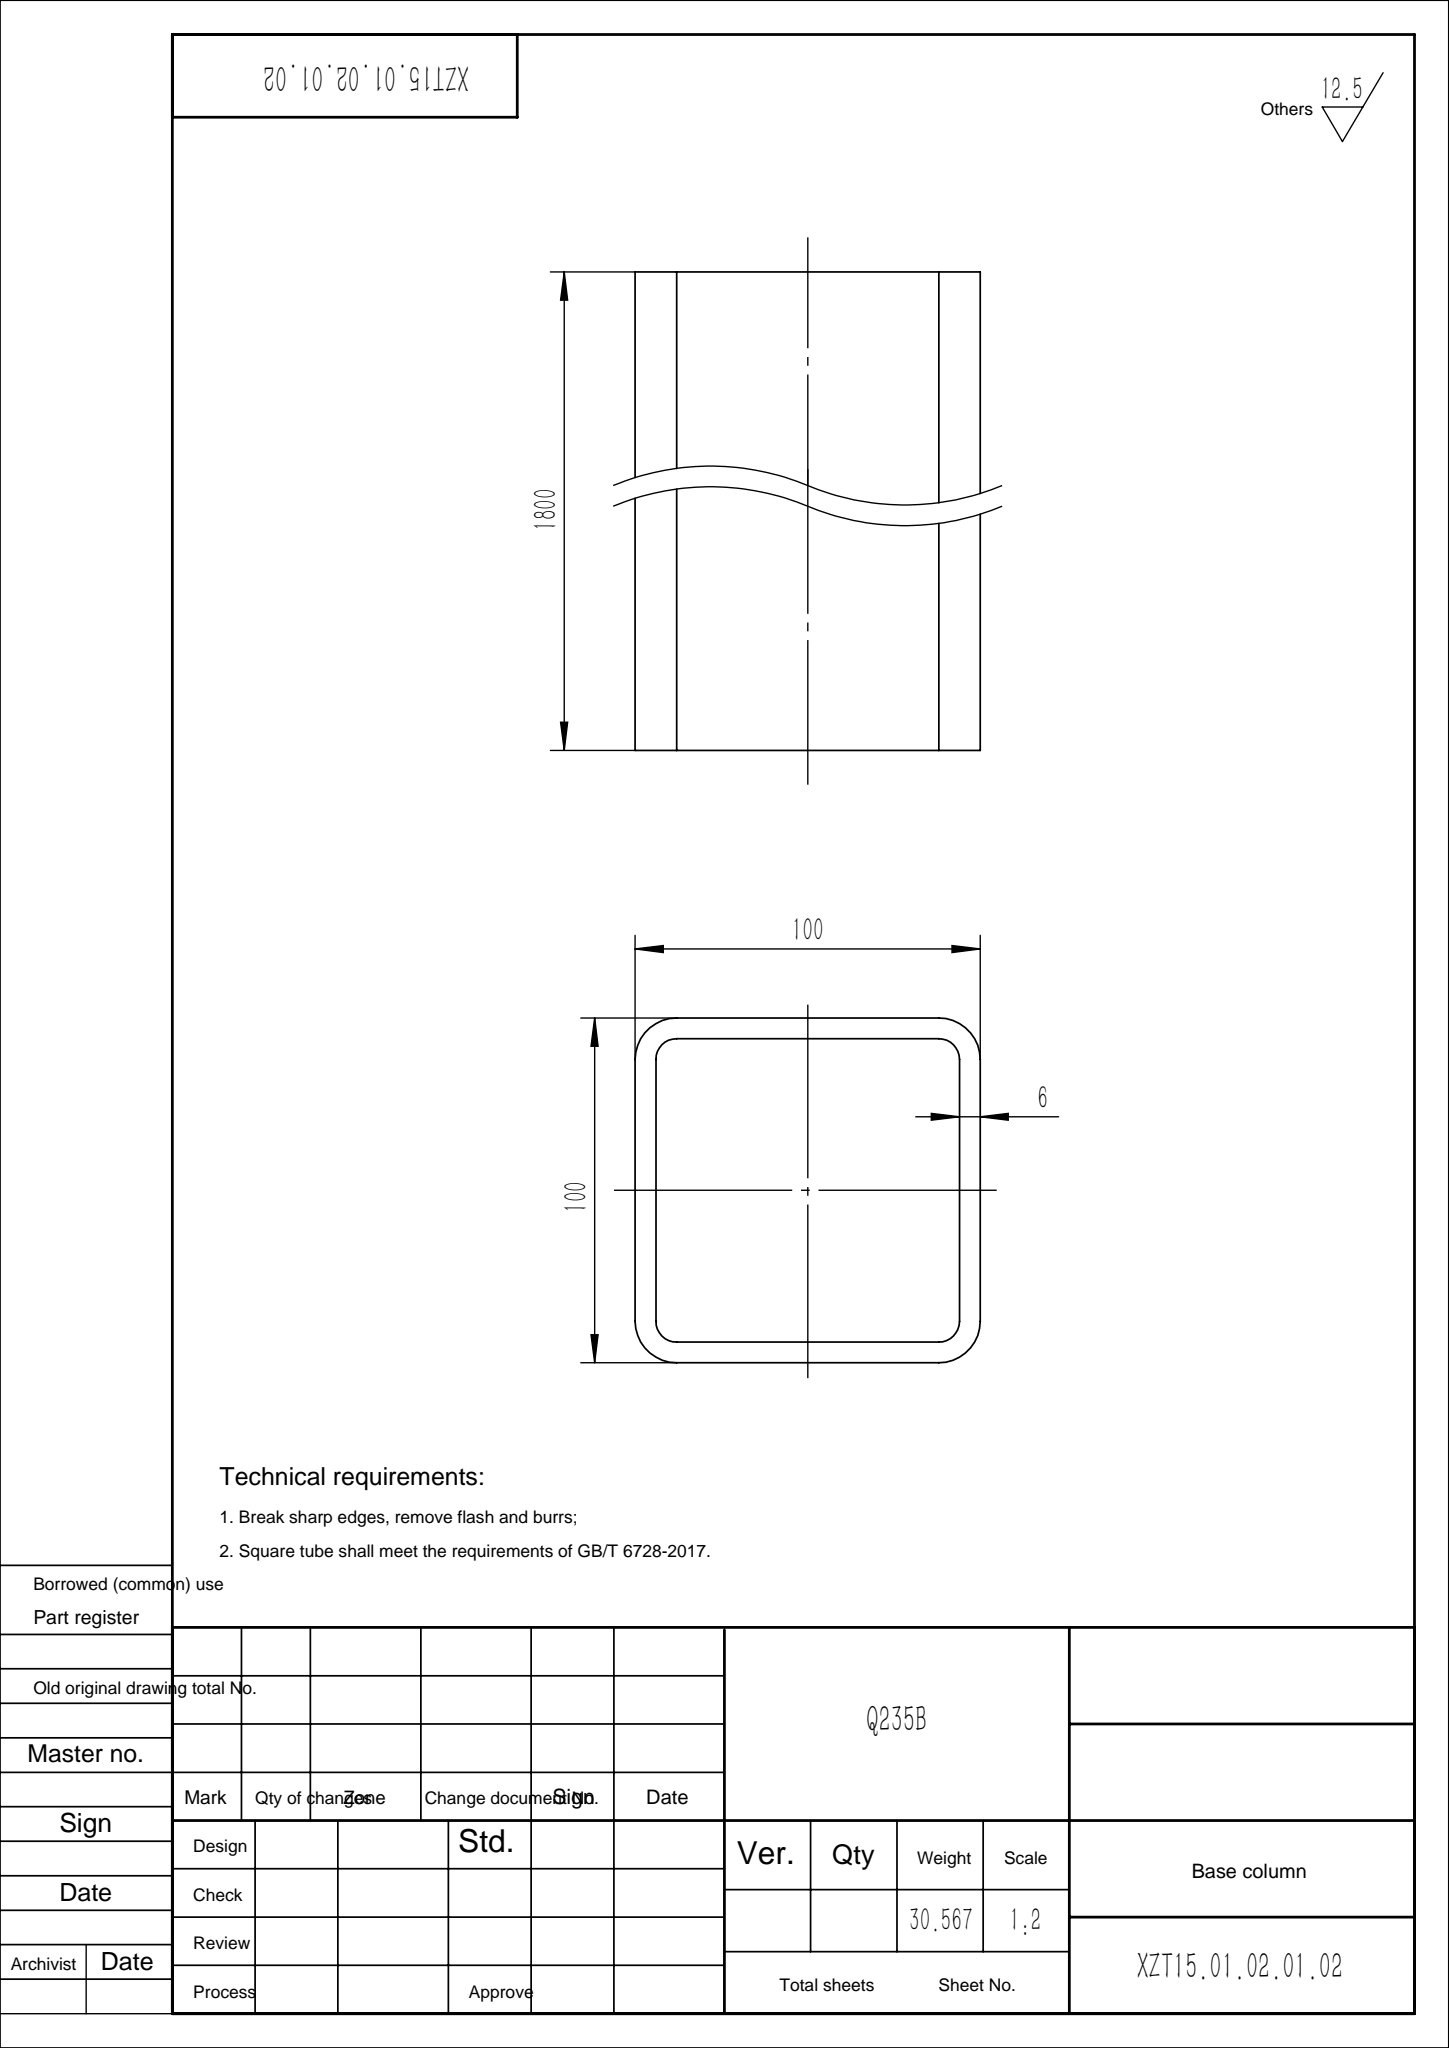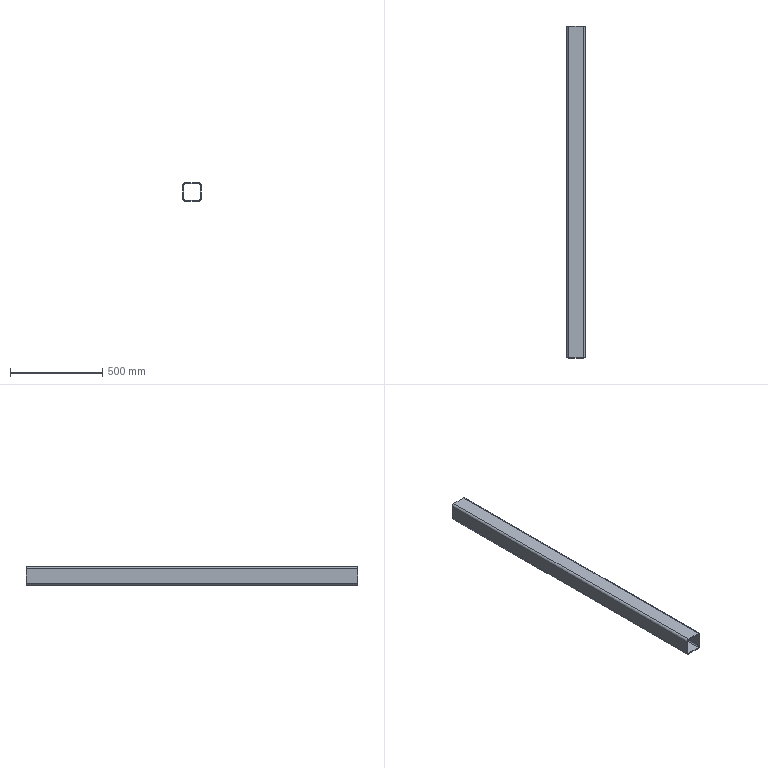Part | SolidWorks | features WeldMemberFeat 1, WeldmentFeature 1 | 1 solid | 18 faces | box 100 x 1800 x 100 mm | volume 3893926 mm3 | plane 10 | cylinder 8 | commonest cylinder face diameters 12 x4 24 x4
STEP:
#1=CARTESIAN_POINT('',(-50.,0.,38.));
#2=VERTEX_POINT('',#1);
#3=CARTESIAN_POINT('',(-38.,0.,50.));
#4=VERTEX_POINT('',#3);
#5=CARTESIAN_POINT('',(-38.,0.,38.));
#6=DIRECTION('',(0.,1.,0.));
#7=DIRECTION('',(0.,0.,1.));
#8=AXIS2_PLACEMENT_3D('',#5,#6,#7);
#9=CIRCLE('',#8,12.);
#10=EDGE_CURVE('',#2,#4,#9,.T.);
#11=ORIENTED_EDGE('',*,*,#10,.T.);
#12=CARTESIAN_POINT('',(-38.,1800.,50.));
#13=VERTEX_POINT('',#12);
#14=CARTESIAN_POINT('',(-38.,1800.,50.));
#15=DIRECTION('',(0.,-1.,0.));
#16=VECTOR('',#15,1000.);
#17=LINE('',#14,#16);
#18=EDGE_CURVE('',#13,#4,#17,.T.);
#19=ORIENTED_EDGE('',*,*,#18,.F.);
#20=CARTESIAN_POINT('',(-50.,1800.,38.));
#21=VERTEX_POINT('',#20);
#22=CARTESIAN_POINT('',(-38.,1800.,38.));
#23=DIRECTION('',(0.,1.,0.));
#24=DIRECTION('',(0.,0.,1.));
#25=AXIS2_PLACEMENT_3D('',#22,#23,#24);
#26=CIRCLE('',#25,12.);
#27=EDGE_CURVE('',#21,#13,#26,.T.);
#28=ORIENTED_EDGE('',*,*,#27,.F.);
#29=CARTESIAN_POINT('',(-50.,1800.,38.));
#30=DIRECTION('',(0.,-1.,0.));
#31=VECTOR('',#30,1000.);
#32=LINE('',#29,#31);
#33=EDGE_CURVE('',#21,#2,#32,.T.);
#34=ORIENTED_EDGE('',*,*,#33,.T.);
#35=EDGE_LOOP('',(#11,#19,#28,#34));
#36=FACE_OUTER_BOUND('',#35,.T.);
#37=CARTESIAN_POINT('',(-38.,1800.,38.));
#38=DIRECTION('',(0.,-1.,0.));
#39=DIRECTION('',(0.,0.,-1.));
#40=AXIS2_PLACEMENT_3D('',#37,#38,#39);
#41=CYLINDRICAL_SURFACE('',#40,12.);
#42=ADVANCED_FACE('',(#36),#41,.T.);
#43=CARTESIAN_POINT('',(38.,0.,50.));
#44=VERTEX_POINT('',#43);
#45=CARTESIAN_POINT('',(-38.,0.,50.));
#46=DIRECTION('',(1.,0.,0.));
#47=VECTOR('',#46,1000.);
#48=LINE('',#45,#47);
#49=EDGE_CURVE('',#4,#44,#48,.T.);
#50=ORIENTED_EDGE('',*,*,#49,.T.);
#51=CARTESIAN_POINT('',(38.,1800.,50.));
#52=VERTEX_POINT('',#51);
#53=CARTESIAN_POINT('',(38.,1800.,50.));
#54=DIRECTION('',(0.,-1.,0.));
#55=VECTOR('',#54,1000.);
#56=LINE('',#53,#55);
#57=EDGE_CURVE('',#52,#44,#56,.T.);
#58=ORIENTED_EDGE('',*,*,#57,.F.);
#59=CARTESIAN_POINT('',(-38.,1800.,50.));
#60=DIRECTION('',(1.,0.,0.));
#61=VECTOR('',#60,1000.);
#62=LINE('',#59,#61);
#63=EDGE_CURVE('',#13,#52,#62,.T.);
#64=ORIENTED_EDGE('',*,*,#63,.F.);
#65=ORIENTED_EDGE('',*,*,#18,.T.);
#66=EDGE_LOOP('',(#50,#58,#64,#65));
#67=FACE_OUTER_BOUND('',#66,.T.);
#68=CARTESIAN_POINT('',(-38.,1800.,50.));
#69=DIRECTION('',(0.,0.,-1.));
#70=DIRECTION('',(-1.,0.,0.));
#71=AXIS2_PLACEMENT_3D('',#68,#69,#70);
#72=PLANE('',#71);
#73=ADVANCED_FACE('',(#67),#72,.F.);
#74=CARTESIAN_POINT('',(50.,0.,38.));
#75=VERTEX_POINT('',#74);
#76=CARTESIAN_POINT('',(38.,0.,38.));
#77=DIRECTION('',(0.,1.,0.));
#78=DIRECTION('',(0.,0.,1.));
#79=AXIS2_PLACEMENT_3D('',#76,#77,#78);
#80=CIRCLE('',#79,12.);
#81=EDGE_CURVE('',#44,#75,#80,.T.);
#82=ORIENTED_EDGE('',*,*,#81,.T.);
#83=CARTESIAN_POINT('',(50.,1800.,38.));
#84=VERTEX_POINT('',#83);
#85=CARTESIAN_POINT('',(50.,1800.,38.));
#86=DIRECTION('',(0.,-1.,0.));
#87=VECTOR('',#86,1000.);
#88=LINE('',#85,#87);
#89=EDGE_CURVE('',#84,#75,#88,.T.);
#90=ORIENTED_EDGE('',*,*,#89,.F.);
#91=CARTESIAN_POINT('',(38.,1800.,38.));
#92=DIRECTION('',(0.,1.,0.));
#93=DIRECTION('',(0.,0.,1.));
#94=AXIS2_PLACEMENT_3D('',#91,#92,#93);
#95=CIRCLE('',#94,12.);
#96=EDGE_CURVE('',#52,#84,#95,.T.);
#97=ORIENTED_EDGE('',*,*,#96,.F.);
#98=ORIENTED_EDGE('',*,*,#57,.T.);
#99=EDGE_LOOP('',(#82,#90,#97,#98));
#100=FACE_OUTER_BOUND('',#99,.T.);
#101=CARTESIAN_POINT('',(38.,1800.,38.));
#102=DIRECTION('',(0.,-1.,0.));
#103=DIRECTION('',(0.,0.,-1.));
#104=AXIS2_PLACEMENT_3D('',#101,#102,#103);
#105=CYLINDRICAL_SURFACE('',#104,12.);
#106=ADVANCED_FACE('',(#100),#105,.T.);
#107=CARTESIAN_POINT('',(50.,0.,-38.));
#108=VERTEX_POINT('',#107);
#109=CARTESIAN_POINT('',(50.,0.,-38.));
#110=DIRECTION('',(0.,0.,-1.));
#111=VECTOR('',#110,1000.);
#112=LINE('',#109,#111);
#113=EDGE_CURVE('',#75,#108,#112,.T.);
#114=ORIENTED_EDGE('',*,*,#113,.T.);
#115=CARTESIAN_POINT('',(50.,1800.,-38.));
#116=VERTEX_POINT('',#115);
#117=CARTESIAN_POINT('',(50.,1800.,-38.));
#118=DIRECTION('',(0.,-1.,0.));
#119=VECTOR('',#118,1000.);
#120=LINE('',#117,#119);
#121=EDGE_CURVE('',#116,#108,#120,.T.);
#122=ORIENTED_EDGE('',*,*,#121,.F.);
#123=CARTESIAN_POINT('',(50.,1800.,-38.));
#124=DIRECTION('',(0.,0.,-1.));
#125=VECTOR('',#124,1000.);
#126=LINE('',#123,#125);
#127=EDGE_CURVE('',#84,#116,#126,.T.);
#128=ORIENTED_EDGE('',*,*,#127,.F.);
#129=ORIENTED_EDGE('',*,*,#89,.T.);
#130=EDGE_LOOP('',(#114,#122,#128,#129));
#131=FACE_OUTER_BOUND('',#130,.T.);
#132=CARTESIAN_POINT('',(50.,1800.,-38.));
#133=DIRECTION('',(-1.,0.,0.));
#134=DIRECTION('',(0.,0.,1.));
#135=AXIS2_PLACEMENT_3D('',#132,#133,#134);
#136=PLANE('',#135);
#137=ADVANCED_FACE('',(#131),#136,.F.);
#138=CARTESIAN_POINT('',(38.,0.,-50.));
#139=VERTEX_POINT('',#138);
#140=CARTESIAN_POINT('',(38.,0.,-38.));
#141=DIRECTION('',(0.,1.,0.));
#142=DIRECTION('',(0.,0.,1.));
#143=AXIS2_PLACEMENT_3D('',#140,#141,#142);
#144=CIRCLE('',#143,12.);
#145=EDGE_CURVE('',#108,#139,#144,.T.);
#146=ORIENTED_EDGE('',*,*,#145,.T.);
#147=CARTESIAN_POINT('',(38.,1800.,-50.));
#148=VERTEX_POINT('',#147);
#149=CARTESIAN_POINT('',(38.,1800.,-50.));
#150=DIRECTION('',(0.,-1.,0.));
#151=VECTOR('',#150,1000.);
#152=LINE('',#149,#151);
#153=EDGE_CURVE('',#148,#139,#152,.T.);
#154=ORIENTED_EDGE('',*,*,#153,.F.);
#155=CARTESIAN_POINT('',(38.,1800.,-38.));
#156=DIRECTION('',(0.,1.,0.));
#157=DIRECTION('',(0.,0.,1.));
#158=AXIS2_PLACEMENT_3D('',#155,#156,#157);
#159=CIRCLE('',#158,12.);
#160=EDGE_CURVE('',#116,#148,#159,.T.);
#161=ORIENTED_EDGE('',*,*,#160,.F.);
#162=ORIENTED_EDGE('',*,*,#121,.T.);
#163=EDGE_LOOP('',(#146,#154,#161,#162));
#164=FACE_OUTER_BOUND('',#163,.T.);
#165=CARTESIAN_POINT('',(38.,1800.,-38.));
#166=DIRECTION('',(0.,-1.,0.));
#167=DIRECTION('',(0.,0.,-1.));
#168=AXIS2_PLACEMENT_3D('',#165,#166,#167);
#169=CYLINDRICAL_SURFACE('',#168,12.);
#170=ADVANCED_FACE('',(#164),#169,.T.);
#171=CARTESIAN_POINT('',(-38.,0.,-50.));
#172=VERTEX_POINT('',#171);
#173=CARTESIAN_POINT('',(38.,0.,-50.));
#174=DIRECTION('',(-1.,0.,0.));
#175=VECTOR('',#174,1000.);
#176=LINE('',#173,#175);
#177=EDGE_CURVE('',#139,#172,#176,.T.);
#178=ORIENTED_EDGE('',*,*,#177,.T.);
#179=CARTESIAN_POINT('',(-38.,1800.,-50.));
#180=VERTEX_POINT('',#179);
#181=CARTESIAN_POINT('',(-38.,1800.,-50.));
#182=DIRECTION('',(0.,-1.,0.));
#183=VECTOR('',#182,1000.);
#184=LINE('',#181,#183);
#185=EDGE_CURVE('',#180,#172,#184,.T.);
#186=ORIENTED_EDGE('',*,*,#185,.F.);
#187=CARTESIAN_POINT('',(38.,1800.,-50.));
#188=DIRECTION('',(-1.,0.,0.));
#189=VECTOR('',#188,1000.);
#190=LINE('',#187,#189);
#191=EDGE_CURVE('',#148,#180,#190,.T.);
#192=ORIENTED_EDGE('',*,*,#191,.F.);
#193=ORIENTED_EDGE('',*,*,#153,.T.);
#194=EDGE_LOOP('',(#178,#186,#192,#193));
#195=FACE_OUTER_BOUND('',#194,.T.);
#196=CARTESIAN_POINT('',(38.,1800.,-50.));
#197=DIRECTION('',(0.,0.,1.));
#198=DIRECTION('',(1.,0.,0.));
#199=AXIS2_PLACEMENT_3D('',#196,#197,#198);
#200=PLANE('',#199);
#201=ADVANCED_FACE('',(#195),#200,.F.);
#202=CARTESIAN_POINT('',(-50.,0.,-38.));
#203=VERTEX_POINT('',#202);
#204=CARTESIAN_POINT('',(-38.,0.,-38.));
#205=DIRECTION('',(0.,1.,0.));
#206=DIRECTION('',(0.,0.,1.));
#207=AXIS2_PLACEMENT_3D('',#204,#205,#206);
#208=CIRCLE('',#207,12.);
#209=EDGE_CURVE('',#172,#203,#208,.T.);
#210=ORIENTED_EDGE('',*,*,#209,.T.);
#211=CARTESIAN_POINT('',(-50.,1800.,-38.));
#212=VERTEX_POINT('',#211);
#213=CARTESIAN_POINT('',(-50.,1800.,-38.));
#214=DIRECTION('',(0.,-1.,0.));
#215=VECTOR('',#214,1000.);
#216=LINE('',#213,#215);
#217=EDGE_CURVE('',#212,#203,#216,.T.);
#218=ORIENTED_EDGE('',*,*,#217,.F.);
#219=CARTESIAN_POINT('',(-38.,1800.,-38.));
#220=DIRECTION('',(0.,1.,0.));
#221=DIRECTION('',(0.,0.,1.));
#222=AXIS2_PLACEMENT_3D('',#219,#220,#221);
#223=CIRCLE('',#222,12.);
#224=EDGE_CURVE('',#180,#212,#223,.T.);
#225=ORIENTED_EDGE('',*,*,#224,.F.);
#226=ORIENTED_EDGE('',*,*,#185,.T.);
#227=EDGE_LOOP('',(#210,#218,#225,#226));
#228=FACE_OUTER_BOUND('',#227,.T.);
#229=CARTESIAN_POINT('',(-38.,1800.,-38.));
#230=DIRECTION('',(0.,-1.,0.));
#231=DIRECTION('',(0.,0.,-1.));
#232=AXIS2_PLACEMENT_3D('',#229,#230,#231);
#233=CYLINDRICAL_SURFACE('',#232,12.);
#234=ADVANCED_FACE('',(#228),#233,.T.);
#235=CARTESIAN_POINT('',(38.,0.,44.));
#236=VERTEX_POINT('',#235);
#237=CARTESIAN_POINT('',(44.,0.,38.));
#238=VERTEX_POINT('',#237);
#239=CARTESIAN_POINT('',(38.,0.,38.));
#240=DIRECTION('',(0.,1.,0.));
#241=DIRECTION('',(0.,0.,1.));
#242=AXIS2_PLACEMENT_3D('',#239,#240,#241);
#243=CIRCLE('',#242,6.);
#244=EDGE_CURVE('',#236,#238,#243,.T.);
#245=ORIENTED_EDGE('',*,*,#244,.F.);
#246=CARTESIAN_POINT('',(38.,1800.,44.));
#247=VERTEX_POINT('',#246);
#248=CARTESIAN_POINT('',(38.,1800.,44.));
#249=DIRECTION('',(0.,-1.,0.));
#250=VECTOR('',#249,1000.);
#251=LINE('',#248,#250);
#252=EDGE_CURVE('',#247,#236,#251,.T.);
#253=ORIENTED_EDGE('',*,*,#252,.F.);
#254=CARTESIAN_POINT('',(44.,1800.,38.));
#255=VERTEX_POINT('',#254);
#256=CARTESIAN_POINT('',(38.,1800.,38.));
#257=DIRECTION('',(0.,1.,0.));
#258=DIRECTION('',(0.,0.,1.));
#259=AXIS2_PLACEMENT_3D('',#256,#257,#258);
#260=CIRCLE('',#259,6.);
#261=EDGE_CURVE('',#247,#255,#260,.T.);
#262=ORIENTED_EDGE('',*,*,#261,.T.);
#263=CARTESIAN_POINT('',(44.,1800.,38.));
#264=DIRECTION('',(0.,-1.,0.));
#265=VECTOR('',#264,1000.);
#266=LINE('',#263,#265);
#267=EDGE_CURVE('',#255,#238,#266,.T.);
#268=ORIENTED_EDGE('',*,*,#267,.T.);
#269=EDGE_LOOP('',(#245,#253,#262,#268));
#270=FACE_OUTER_BOUND('',#269,.T.);
#271=CARTESIAN_POINT('',(38.,1800.,38.));
#272=DIRECTION('',(0.,-1.,0.));
#273=DIRECTION('',(0.,0.,-1.));
#274=AXIS2_PLACEMENT_3D('',#271,#272,#273);
#275=CYLINDRICAL_SURFACE('',#274,6.);
#276=ADVANCED_FACE('',(#270),#275,.F.);
#277=CARTESIAN_POINT('',(-38.,0.,44.));
#278=VERTEX_POINT('',#277);
#279=CARTESIAN_POINT('',(-38.,0.,44.));
#280=DIRECTION('',(1.,0.,0.));
#281=VECTOR('',#280,1000.);
#282=LINE('',#279,#281);
#283=EDGE_CURVE('',#278,#236,#282,.T.);
#284=ORIENTED_EDGE('',*,*,#283,.F.);
#285=CARTESIAN_POINT('',(-38.,1800.,44.));
#286=VERTEX_POINT('',#285);
#287=CARTESIAN_POINT('',(-38.,1800.,44.));
#288=DIRECTION('',(0.,-1.,0.));
#289=VECTOR('',#288,1000.);
#290=LINE('',#287,#289);
#291=EDGE_CURVE('',#286,#278,#290,.T.);
#292=ORIENTED_EDGE('',*,*,#291,.F.);
#293=CARTESIAN_POINT('',(-38.,1800.,44.));
#294=DIRECTION('',(1.,0.,0.));
#295=VECTOR('',#294,1000.);
#296=LINE('',#293,#295);
#297=EDGE_CURVE('',#286,#247,#296,.T.);
#298=ORIENTED_EDGE('',*,*,#297,.T.);
#299=ORIENTED_EDGE('',*,*,#252,.T.);
#300=EDGE_LOOP('',(#284,#292,#298,#299));
#301=FACE_OUTER_BOUND('',#300,.T.);
#302=CARTESIAN_POINT('',(-38.,1800.,44.));
#303=DIRECTION('',(0.,0.,-1.));
#304=DIRECTION('',(-1.,0.,0.));
#305=AXIS2_PLACEMENT_3D('',#302,#303,#304);
#306=PLANE('',#305);
#307=ADVANCED_FACE('',(#301),#306,.T.);
#308=CARTESIAN_POINT('',(-44.,0.,38.));
#309=VERTEX_POINT('',#308);
#310=CARTESIAN_POINT('',(-38.,0.,38.));
#311=DIRECTION('',(0.,1.,0.));
#312=DIRECTION('',(0.,0.,1.));
#313=AXIS2_PLACEMENT_3D('',#310,#311,#312);
#314=CIRCLE('',#313,6.);
#315=EDGE_CURVE('',#309,#278,#314,.T.);
#316=ORIENTED_EDGE('',*,*,#315,.F.);
#317=CARTESIAN_POINT('',(-44.,1800.,38.));
#318=VERTEX_POINT('',#317);
#319=CARTESIAN_POINT('',(-44.,1800.,38.));
#320=DIRECTION('',(0.,-1.,0.));
#321=VECTOR('',#320,1000.);
#322=LINE('',#319,#321);
#323=EDGE_CURVE('',#318,#309,#322,.T.);
#324=ORIENTED_EDGE('',*,*,#323,.F.);
#325=CARTESIAN_POINT('',(-38.,1800.,38.));
#326=DIRECTION('',(0.,1.,0.));
#327=DIRECTION('',(0.,0.,1.));
#328=AXIS2_PLACEMENT_3D('',#325,#326,#327);
#329=CIRCLE('',#328,6.);
#330=EDGE_CURVE('',#318,#286,#329,.T.);
#331=ORIENTED_EDGE('',*,*,#330,.T.);
#332=ORIENTED_EDGE('',*,*,#291,.T.);
#333=EDGE_LOOP('',(#316,#324,#331,#332));
#334=FACE_OUTER_BOUND('',#333,.T.);
#335=CARTESIAN_POINT('',(-38.,1800.,38.));
#336=DIRECTION('',(0.,-1.,0.));
#337=DIRECTION('',(0.,0.,-1.));
#338=AXIS2_PLACEMENT_3D('',#335,#336,#337);
#339=CYLINDRICAL_SURFACE('',#338,6.);
#340=ADVANCED_FACE('',(#334),#339,.F.);
#341=CARTESIAN_POINT('',(-44.,0.,-38.));
#342=VERTEX_POINT('',#341);
#343=CARTESIAN_POINT('',(-44.,0.,38.));
#344=DIRECTION('',(0.,0.,1.));
#345=VECTOR('',#344,1000.);
#346=LINE('',#343,#345);
#347=EDGE_CURVE('',#342,#309,#346,.T.);
#348=ORIENTED_EDGE('',*,*,#347,.F.);
#349=CARTESIAN_POINT('',(-44.,1800.,-38.));
#350=VERTEX_POINT('',#349);
#351=CARTESIAN_POINT('',(-44.,1800.,-38.));
#352=DIRECTION('',(0.,-1.,0.));
#353=VECTOR('',#352,1000.);
#354=LINE('',#351,#353);
#355=EDGE_CURVE('',#350,#342,#354,.T.);
#356=ORIENTED_EDGE('',*,*,#355,.F.);
#357=CARTESIAN_POINT('',(-44.,1800.,38.));
#358=DIRECTION('',(0.,0.,1.));
#359=VECTOR('',#358,1000.);
#360=LINE('',#357,#359);
#361=EDGE_CURVE('',#350,#318,#360,.T.);
#362=ORIENTED_EDGE('',*,*,#361,.T.);
#363=ORIENTED_EDGE('',*,*,#323,.T.);
#364=EDGE_LOOP('',(#348,#356,#362,#363));
#365=FACE_OUTER_BOUND('',#364,.T.);
#366=CARTESIAN_POINT('',(-44.,1800.,38.));
#367=DIRECTION('',(1.,0.,0.));
#368=DIRECTION('',(0.,0.,-1.));
#369=AXIS2_PLACEMENT_3D('',#366,#367,#368);
#370=PLANE('',#369);
#371=ADVANCED_FACE('',(#365),#370,.T.);
#372=CARTESIAN_POINT('',(-38.,0.,-44.));
#373=VERTEX_POINT('',#372);
#374=CARTESIAN_POINT('',(-38.,0.,-38.));
#375=DIRECTION('',(0.,1.,0.));
#376=DIRECTION('',(0.,0.,1.));
#377=AXIS2_PLACEMENT_3D('',#374,#375,#376);
#378=CIRCLE('',#377,6.);
#379=EDGE_CURVE('',#373,#342,#378,.T.);
#380=ORIENTED_EDGE('',*,*,#379,.F.);
#381=CARTESIAN_POINT('',(-38.,1800.,-44.));
#382=VERTEX_POINT('',#381);
#383=CARTESIAN_POINT('',(-38.,1800.,-44.));
#384=DIRECTION('',(0.,-1.,0.));
#385=VECTOR('',#384,1000.);
#386=LINE('',#383,#385);
#387=EDGE_CURVE('',#382,#373,#386,.T.);
#388=ORIENTED_EDGE('',*,*,#387,.F.);
#389=CARTESIAN_POINT('',(-38.,1800.,-38.));
#390=DIRECTION('',(0.,1.,0.));
#391=DIRECTION('',(0.,0.,1.));
#392=AXIS2_PLACEMENT_3D('',#389,#390,#391);
#393=CIRCLE('',#392,6.);
#394=EDGE_CURVE('',#382,#350,#393,.T.);
#395=ORIENTED_EDGE('',*,*,#394,.T.);
#396=ORIENTED_EDGE('',*,*,#355,.T.);
#397=EDGE_LOOP('',(#380,#388,#395,#396));
#398=FACE_OUTER_BOUND('',#397,.T.);
#399=CARTESIAN_POINT('',(-38.,1800.,-38.));
#400=DIRECTION('',(0.,-1.,0.));
#401=DIRECTION('',(0.,0.,-1.));
#402=AXIS2_PLACEMENT_3D('',#399,#400,#401);
#403=CYLINDRICAL_SURFACE('',#402,6.);
#404=ADVANCED_FACE('',(#398),#403,.F.);
#405=CARTESIAN_POINT('',(38.,0.,-44.));
#406=VERTEX_POINT('',#405);
#407=CARTESIAN_POINT('',(38.,0.,-44.));
#408=DIRECTION('',(-1.,0.,0.));
#409=VECTOR('',#408,1000.);
#410=LINE('',#407,#409);
#411=EDGE_CURVE('',#406,#373,#410,.T.);
#412=ORIENTED_EDGE('',*,*,#411,.F.);
#413=CARTESIAN_POINT('',(38.,1800.,-44.));
#414=VERTEX_POINT('',#413);
#415=CARTESIAN_POINT('',(38.,1800.,-44.));
#416=DIRECTION('',(0.,-1.,0.));
#417=VECTOR('',#416,1000.);
#418=LINE('',#415,#417);
#419=EDGE_CURVE('',#414,#406,#418,.T.);
#420=ORIENTED_EDGE('',*,*,#419,.F.);
#421=CARTESIAN_POINT('',(38.,1800.,-44.));
#422=DIRECTION('',(-1.,0.,0.));
#423=VECTOR('',#422,1000.);
#424=LINE('',#421,#423);
#425=EDGE_CURVE('',#414,#382,#424,.T.);
#426=ORIENTED_EDGE('',*,*,#425,.T.);
#427=ORIENTED_EDGE('',*,*,#387,.T.);
#428=EDGE_LOOP('',(#412,#420,#426,#427));
#429=FACE_OUTER_BOUND('',#428,.T.);
#430=CARTESIAN_POINT('',(38.,1800.,-44.));
#431=DIRECTION('',(0.,0.,1.));
#432=DIRECTION('',(1.,0.,0.));
#433=AXIS2_PLACEMENT_3D('',#430,#431,#432);
#434=PLANE('',#433);
#435=ADVANCED_FACE('',(#429),#434,.T.);
#436=CARTESIAN_POINT('',(44.,0.,-38.));
#437=VERTEX_POINT('',#436);
#438=CARTESIAN_POINT('',(38.,0.,-38.));
#439=DIRECTION('',(0.,1.,0.));
#440=DIRECTION('',(0.,0.,1.));
#441=AXIS2_PLACEMENT_3D('',#438,#439,#440);
#442=CIRCLE('',#441,6.);
#443=EDGE_CURVE('',#437,#406,#442,.T.);
#444=ORIENTED_EDGE('',*,*,#443,.F.);
#445=CARTESIAN_POINT('',(44.,1800.,-38.));
#446=VERTEX_POINT('',#445);
#447=CARTESIAN_POINT('',(44.,1800.,-38.));
#448=DIRECTION('',(0.,-1.,0.));
#449=VECTOR('',#448,1000.);
#450=LINE('',#447,#449);
#451=EDGE_CURVE('',#446,#437,#450,.T.);
#452=ORIENTED_EDGE('',*,*,#451,.F.);
#453=CARTESIAN_POINT('',(38.,1800.,-38.));
#454=DIRECTION('',(0.,1.,0.));
#455=DIRECTION('',(0.,0.,1.));
#456=AXIS2_PLACEMENT_3D('',#453,#454,#455);
#457=CIRCLE('',#456,6.);
#458=EDGE_CURVE('',#446,#414,#457,.T.);
#459=ORIENTED_EDGE('',*,*,#458,.T.);
#460=ORIENTED_EDGE('',*,*,#419,.T.);
#461=EDGE_LOOP('',(#444,#452,#459,#460));
#462=FACE_OUTER_BOUND('',#461,.T.);
#463=CARTESIAN_POINT('',(38.,1800.,-38.));
#464=DIRECTION('',(0.,-1.,0.));
#465=DIRECTION('',(0.,0.,-1.));
#466=AXIS2_PLACEMENT_3D('',#463,#464,#465);
#467=CYLINDRICAL_SURFACE('',#466,6.);
#468=ADVANCED_FACE('',(#462),#467,.F.);
#469=CARTESIAN_POINT('',(44.,0.,-38.));
#470=DIRECTION('',(0.,0.,-1.));
#471=VECTOR('',#470,1000.);
#472=LINE('',#469,#471);
#473=EDGE_CURVE('',#238,#437,#472,.T.);
#474=ORIENTED_EDGE('',*,*,#473,.F.);
#475=ORIENTED_EDGE('',*,*,#267,.F.);
#476=CARTESIAN_POINT('',(44.,1800.,-38.));
#477=DIRECTION('',(0.,0.,-1.));
#478=VECTOR('',#477,1000.);
#479=LINE('',#476,#478);
#480=EDGE_CURVE('',#255,#446,#479,.T.);
#481=ORIENTED_EDGE('',*,*,#480,.T.);
#482=ORIENTED_EDGE('',*,*,#451,.T.);
#483=EDGE_LOOP('',(#474,#475,#481,#482));
#484=FACE_OUTER_BOUND('',#483,.T.);
#485=CARTESIAN_POINT('',(44.,1800.,-38.));
#486=DIRECTION('',(-1.,0.,0.));
#487=DIRECTION('',(0.,0.,1.));
#488=AXIS2_PLACEMENT_3D('',#485,#486,#487);
#489=PLANE('',#488);
#490=ADVANCED_FACE('',(#484),#489,.T.);
#491=CARTESIAN_POINT('',(-50.,0.,38.));
#492=DIRECTION('',(0.,0.,1.));
#493=VECTOR('',#492,1000.);
#494=LINE('',#491,#493);
#495=EDGE_CURVE('',#203,#2,#494,.T.);
#496=ORIENTED_EDGE('',*,*,#495,.T.);
#497=ORIENTED_EDGE('',*,*,#33,.F.);
#498=CARTESIAN_POINT('',(-50.,1800.,38.));
#499=DIRECTION('',(0.,0.,1.));
#500=VECTOR('',#499,1000.);
#501=LINE('',#498,#500);
#502=EDGE_CURVE('',#212,#21,#501,.T.);
#503=ORIENTED_EDGE('',*,*,#502,.F.);
#504=ORIENTED_EDGE('',*,*,#217,.T.);
#505=EDGE_LOOP('',(#496,#497,#503,#504));
#506=FACE_OUTER_BOUND('',#505,.T.);
#507=CARTESIAN_POINT('',(-50.,1800.,38.));
#508=DIRECTION('',(1.,0.,0.));
#509=DIRECTION('',(0.,0.,-1.));
#510=AXIS2_PLACEMENT_3D('',#507,#508,#509);
#511=PLANE('',#510);
#512=ADVANCED_FACE('',(#506),#511,.F.);
#513=ORIENTED_EDGE('',*,*,#261,.F.);
#514=ORIENTED_EDGE('',*,*,#297,.F.);
#515=ORIENTED_EDGE('',*,*,#330,.F.);
#516=ORIENTED_EDGE('',*,*,#361,.F.);
#517=ORIENTED_EDGE('',*,*,#394,.F.);
#518=ORIENTED_EDGE('',*,*,#425,.F.);
#519=ORIENTED_EDGE('',*,*,#458,.F.);
#520=ORIENTED_EDGE('',*,*,#480,.F.);
#521=EDGE_LOOP('',(#513,#514,#515,#516,#517,#518,#519,#520));
#522=FACE_BOUND('',#521,.T.);
#523=ORIENTED_EDGE('',*,*,#27,.T.);
#524=ORIENTED_EDGE('',*,*,#63,.T.);
#525=ORIENTED_EDGE('',*,*,#96,.T.);
#526=ORIENTED_EDGE('',*,*,#127,.T.);
#527=ORIENTED_EDGE('',*,*,#160,.T.);
#528=ORIENTED_EDGE('',*,*,#191,.T.);
#529=ORIENTED_EDGE('',*,*,#224,.T.);
#530=ORIENTED_EDGE('',*,*,#502,.T.);
#531=EDGE_LOOP('',(#523,#524,#525,#526,#527,#528,#529,#530));
#532=FACE_OUTER_BOUND('',#531,.T.);
#533=CARTESIAN_POINT('',(-38.,1800.,38.));
#534=DIRECTION('',(0.,1.,0.));
#535=DIRECTION('',(0.,0.,1.));
#536=AXIS2_PLACEMENT_3D('',#533,#534,#535);
#537=PLANE('',#536);
#538=ADVANCED_FACE('',(#522,#532),#537,.T.);
#539=ORIENTED_EDGE('',*,*,#244,.T.);
#540=ORIENTED_EDGE('',*,*,#473,.T.);
#541=ORIENTED_EDGE('',*,*,#443,.T.);
#542=ORIENTED_EDGE('',*,*,#411,.T.);
#543=ORIENTED_EDGE('',*,*,#379,.T.);
#544=ORIENTED_EDGE('',*,*,#347,.T.);
#545=ORIENTED_EDGE('',*,*,#315,.T.);
#546=ORIENTED_EDGE('',*,*,#283,.T.);
#547=EDGE_LOOP('',(#539,#540,#541,#542,#543,#544,#545,#546));
#548=FACE_BOUND('',#547,.T.);
#549=ORIENTED_EDGE('',*,*,#10,.F.);
#550=ORIENTED_EDGE('',*,*,#495,.F.);
#551=ORIENTED_EDGE('',*,*,#209,.F.);
#552=ORIENTED_EDGE('',*,*,#177,.F.);
#553=ORIENTED_EDGE('',*,*,#145,.F.);
#554=ORIENTED_EDGE('',*,*,#113,.F.);
#555=ORIENTED_EDGE('',*,*,#81,.F.);
#556=ORIENTED_EDGE('',*,*,#49,.F.);
#557=EDGE_LOOP('',(#549,#550,#551,#552,#553,#554,#555,#556));
#558=FACE_OUTER_BOUND('',#557,.T.);
#559=CARTESIAN_POINT('',(-38.,0.,38.));
#560=DIRECTION('',(0.,1.,0.));
#561=DIRECTION('',(0.,0.,1.));
#562=AXIS2_PLACEMENT_3D('',#559,#560,#561);
#563=PLANE('',#562);
#564=ADVANCED_FACE('',(#548,#558),#563,.F.);
#565=CLOSED_SHELL('',(#42,#73,#106,#137,#170,#201,#234,#276,#307,#340,#371,#404,#435,#468,#490,#512,#538,#564));
#566=MANIFOLD_SOLID_BREP('',#565);
#567=CARTESIAN_POINT('',(0.,0.,0.));
#568=DIRECTION('',(0.,0.,1.));
#569=DIRECTION('',(1.,0.,0.));
#570=AXIS2_PLACEMENT_3D('',#567,#568,#569);
#571=(LENGTH_UNIT()NAMED_UNIT(*)SI_UNIT(.MILLI.,.METRE.));
#572=UNCERTAINTY_MEASURE_WITH_UNIT(LENGTH_MEASURE(0.00001),#571,'','');
#573=(NAMED_UNIT(*)PLANE_ANGLE_UNIT()SI_UNIT($,.RADIAN.));
#574=(NAMED_UNIT(*)SI_UNIT($,.STERADIAN.)SOLID_ANGLE_UNIT());
#575=(GEOMETRIC_REPRESENTATION_CONTEXT(3)GLOBAL_UNCERTAINTY_ASSIGNED_CONTEXT((#572))GLOBAL_UNIT_ASSIGNED_CONTEXT((#571,#573,#574))REPRESENTATION_CONTEXT('',''));
#576=ADVANCED_BREP_SHAPE_REPRESENTATION('',(#566,#570),#575);